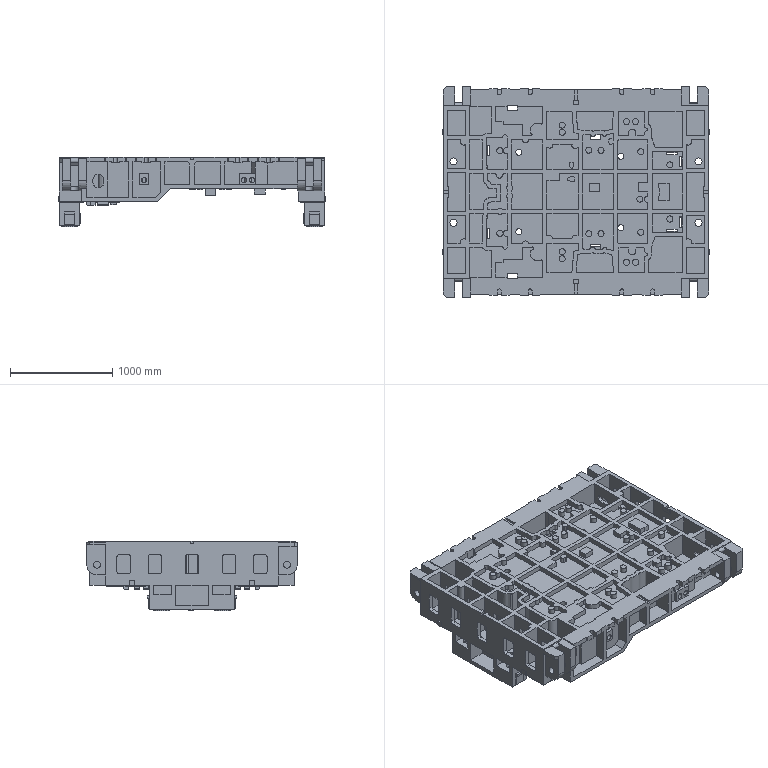Part | NX | features solid 2 | 2 solids | 1686 faces | box 2620 x 2060 x 680 mm | volume 690971108 mm3 | plane 1340 | cylinder 280 | spline 66 | commonest cylinder face diameters 40 x83 60 x76 30 x24 100 x13 70 x12 80 x12